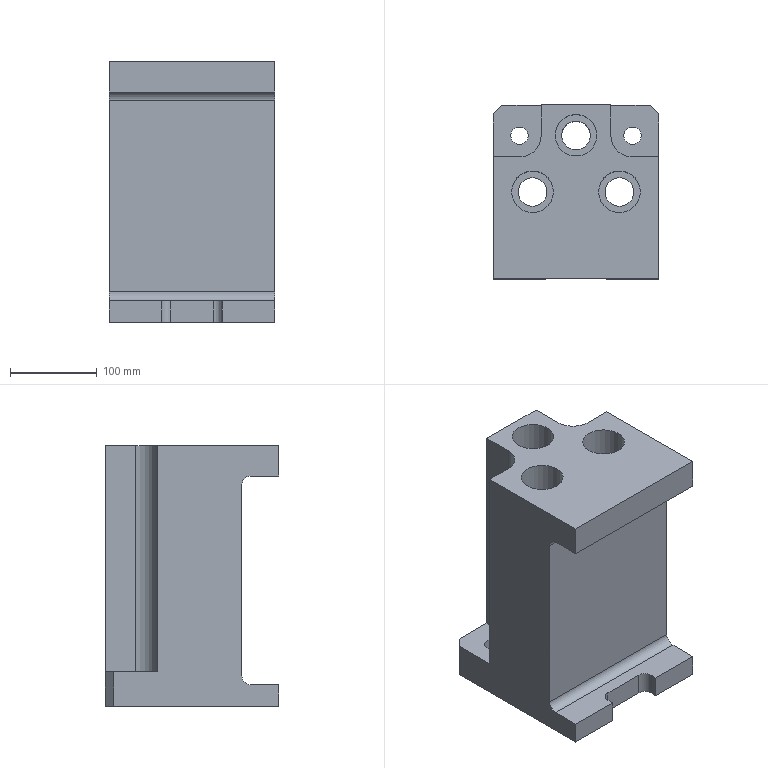Part | NX | features DATUM_CSYS 6, SKETCH 5, EXTRUDE 4, CBORE_HOLE 3, BLEND 2, HOLE PACKAGE 2, SIMPLE HOLE 2, CHAMFER 1 | 1 solid | 39 faces | box 190.5 x 200 x 300 mm | volume 6616630 mm3 | plane 25 | cylinder 14 | commonest cylinder face diameters 20 x6 33 x3 48 x3 50 x2
STEP:
#1=CARTESIAN_POINT('',(-95.25,-100.,0.));
#2=VERTEX_POINT('',#1);
#3=CARTESIAN_POINT('',(-35.,-100.,0.));
#4=VERTEX_POINT('',#3);
#5=CARTESIAN_POINT('',(-95.25,-100.,0.));
#6=DIRECTION('',(1.,0.,0.));
#7=VECTOR('',#6,1000.);
#8=LINE('',#5,#7);
#9=EDGE_CURVE('',#2,#4,#8,.T.);
#10=ORIENTED_EDGE('',*,*,#9,.T.);
#11=CARTESIAN_POINT('',(-35.,-100.,25.));
#12=VERTEX_POINT('',#11);
#13=CARTESIAN_POINT('',(-35.,-100.,300.));
#14=DIRECTION('',(0.,0.,1.));
#15=VECTOR('',#14,1000.);
#16=LINE('',#13,#15);
#17=EDGE_CURVE('',#4,#12,#16,.T.);
#18=ORIENTED_EDGE('',*,*,#17,.T.);
#19=CARTESIAN_POINT('',(-95.25,-100.,25.));
#20=VERTEX_POINT('',#19);
#21=CARTESIAN_POINT('',(-95.25,-100.,25.));
#22=DIRECTION('',(-1.,0.,0.));
#23=VECTOR('',#22,1000.);
#24=LINE('',#21,#23);
#25=EDGE_CURVE('',#12,#20,#24,.T.);
#26=ORIENTED_EDGE('',*,*,#25,.T.);
#27=CARTESIAN_POINT('',(-95.25,-100.,300.));
#28=DIRECTION('',(0.,0.,-1.));
#29=VECTOR('',#28,1000.);
#30=LINE('',#27,#29);
#31=EDGE_CURVE('',#20,#2,#30,.T.);
#32=ORIENTED_EDGE('',*,*,#31,.T.);
#33=EDGE_LOOP('',(#10,#18,#26,#32));
#34=FACE_BOUND('',#33,.T.);
#35=CARTESIAN_POINT('',(-95.25,-100.,300.));
#36=DIRECTION('',(0.,1.,0.));
#37=DIRECTION('',(0.,0.,1.));
#38=AXIS2_PLACEMENT_3D('',#35,#36,#37);
#39=PLANE('',#38);
#40=ADVANCED_FACE('',(#34),#39,.F.);
#41=CARTESIAN_POINT('',(-33.5,0.,0.));
#42=VERTEX_POINT('',#41);
#43=CARTESIAN_POINT('',(-50.,0.,0.));
#44=DIRECTION('',(0.,0.,1.));
#45=DIRECTION('',(1.,0.,0.));
#46=AXIS2_PLACEMENT_3D('',#43,#44,#45);
#47=CIRCLE('',#46,16.5);
#48=EDGE_CURVE('',#42,#42,#47,.T.);
#49=ORIENTED_EDGE('',*,*,#48,.T.);
#50=EDGE_LOOP('',(#49));
#51=FACE_BOUND('',#50,.T.);
#52=CARTESIAN_POINT('',(16.5,65.,0.));
#53=VERTEX_POINT('',#52);
#54=CARTESIAN_POINT('',(0.,65.,0.));
#55=DIRECTION('',(0.,0.,1.));
#56=DIRECTION('',(1.,0.,0.));
#57=AXIS2_PLACEMENT_3D('',#54,#55,#56);
#58=CIRCLE('',#57,16.5);
#59=EDGE_CURVE('',#53,#53,#58,.T.);
#60=ORIENTED_EDGE('',*,*,#59,.T.);
#61=EDGE_LOOP('',(#60));
#62=FACE_BOUND('',#61,.T.);
#63=CARTESIAN_POINT('',(66.5,0.,0.));
#64=VERTEX_POINT('',#63);
#65=CARTESIAN_POINT('',(50.,0.,0.));
#66=DIRECTION('',(0.,0.,1.));
#67=DIRECTION('',(1.,0.,0.));
#68=AXIS2_PLACEMENT_3D('',#65,#66,#67);
#69=CIRCLE('',#68,16.5);
#70=EDGE_CURVE('',#64,#64,#69,.T.);
#71=ORIENTED_EDGE('',*,*,#70,.T.);
#72=EDGE_LOOP('',(#71));
#73=FACE_BOUND('',#72,.T.);
#74=CARTESIAN_POINT('',(-55.,65.,0.));
#75=VERTEX_POINT('',#74);
#76=CARTESIAN_POINT('',(-65.,65.,0.));
#77=DIRECTION('',(0.,0.,1.));
#78=DIRECTION('',(1.,0.,0.));
#79=AXIS2_PLACEMENT_3D('',#76,#77,#78);
#80=CIRCLE('',#79,10.);
#81=EDGE_CURVE('',#75,#75,#80,.T.);
#82=ORIENTED_EDGE('',*,*,#81,.T.);
#83=EDGE_LOOP('',(#82));
#84=FACE_BOUND('',#83,.T.);
#85=CARTESIAN_POINT('',(75.,65.,0.));
#86=VERTEX_POINT('',#85);
#87=CARTESIAN_POINT('',(65.,65.,0.));
#88=DIRECTION('',(0.,0.,1.));
#89=DIRECTION('',(1.,0.,0.));
#90=AXIS2_PLACEMENT_3D('',#87,#88,#89);
#91=CIRCLE('',#90,10.);
#92=EDGE_CURVE('',#86,#86,#91,.T.);
#93=ORIENTED_EDGE('',*,*,#92,.T.);
#94=EDGE_LOOP('',(#93));
#95=FACE_BOUND('',#94,.T.);
#96=CARTESIAN_POINT('',(85.25,100.,0.));
#97=VERTEX_POINT('',#96);
#98=CARTESIAN_POINT('',(-85.25,100.,0.));
#99=VERTEX_POINT('',#98);
#100=CARTESIAN_POINT('',(95.25,100.,0.));
#101=DIRECTION('',(-1.,0.,0.));
#102=VECTOR('',#101,1000.);
#103=LINE('',#100,#102);
#104=EDGE_CURVE('',#97,#99,#103,.T.);
#105=ORIENTED_EDGE('',*,*,#104,.F.);
#106=CARTESIAN_POINT('',(95.25,90.,0.));
#107=VERTEX_POINT('',#106);
#108=CARTESIAN_POINT('',(85.25,100.,0.));
#109=DIRECTION('',(-0.7071,0.7071,0.));
#110=VECTOR('',#109,1000.);
#111=LINE('',#108,#110);
#112=EDGE_CURVE('',#97,#107,#111,.F.);
#113=ORIENTED_EDGE('',*,*,#112,.T.);
#114=CARTESIAN_POINT('',(95.25,-100.,0.));
#115=VERTEX_POINT('',#114);
#116=CARTESIAN_POINT('',(95.25,-100.,0.));
#117=DIRECTION('',(0.,1.,0.));
#118=VECTOR('',#117,1000.);
#119=LINE('',#116,#118);
#120=EDGE_CURVE('',#115,#107,#119,.T.);
#121=ORIENTED_EDGE('',*,*,#120,.F.);
#122=CARTESIAN_POINT('',(35.,-100.,0.));
#123=VERTEX_POINT('',#122);
#124=CARTESIAN_POINT('',(-95.25,-100.,0.));
#125=DIRECTION('',(1.,0.,0.));
#126=VECTOR('',#125,1000.);
#127=LINE('',#124,#126);
#128=EDGE_CURVE('',#123,#115,#127,.T.);
#129=ORIENTED_EDGE('',*,*,#128,.F.);
#130=CARTESIAN_POINT('',(35.,-92.,0.));
#131=VERTEX_POINT('',#130);
#132=CARTESIAN_POINT('',(35.,-82.,0.));
#133=DIRECTION('',(0.,-1.,0.));
#134=VECTOR('',#133,1000.);
#135=LINE('',#132,#134);
#136=EDGE_CURVE('',#131,#123,#135,.T.);
#137=ORIENTED_EDGE('',*,*,#136,.F.);
#138=CARTESIAN_POINT('',(25.,-82.,0.));
#139=VERTEX_POINT('',#138);
#140=CARTESIAN_POINT('',(25.,-92.,0.));
#141=DIRECTION('',(0.,0.,1.));
#142=DIRECTION('',(1.,0.,0.));
#143=AXIS2_PLACEMENT_3D('',#140,#141,#142);
#144=CIRCLE('',#143,10.);
#145=EDGE_CURVE('',#131,#139,#144,.T.);
#146=ORIENTED_EDGE('',*,*,#145,.T.);
#147=CARTESIAN_POINT('',(-25.,-82.,0.));
#148=VERTEX_POINT('',#147);
#149=CARTESIAN_POINT('',(-35.,-82.,0.));
#150=DIRECTION('',(1.,0.,0.));
#151=VECTOR('',#150,1000.);
#152=LINE('',#149,#151);
#153=EDGE_CURVE('',#148,#139,#152,.T.);
#154=ORIENTED_EDGE('',*,*,#153,.F.);
#155=CARTESIAN_POINT('',(-35.,-92.,0.));
#156=VERTEX_POINT('',#155);
#157=CARTESIAN_POINT('',(-25.,-92.,0.));
#158=DIRECTION('',(0.,0.,1.));
#159=DIRECTION('',(1.,0.,0.));
#160=AXIS2_PLACEMENT_3D('',#157,#158,#159);
#161=CIRCLE('',#160,10.);
#162=EDGE_CURVE('',#148,#156,#161,.T.);
#163=ORIENTED_EDGE('',*,*,#162,.T.);
#164=CARTESIAN_POINT('',(-35.,-147.,0.));
#165=DIRECTION('',(0.,1.,0.));
#166=VECTOR('',#165,1000.);
#167=LINE('',#164,#166);
#168=EDGE_CURVE('',#4,#156,#167,.T.);
#169=ORIENTED_EDGE('',*,*,#168,.F.);
#170=ORIENTED_EDGE('',*,*,#9,.F.);
#171=CARTESIAN_POINT('',(-95.25,90.,0.));
#172=VERTEX_POINT('',#171);
#173=CARTESIAN_POINT('',(-95.25,100.,0.));
#174=DIRECTION('',(0.,-1.,0.));
#175=VECTOR('',#174,1000.);
#176=LINE('',#173,#175);
#177=EDGE_CURVE('',#172,#2,#176,.T.);
#178=ORIENTED_EDGE('',*,*,#177,.F.);
#179=CARTESIAN_POINT('',(-95.25,90.,0.));
#180=DIRECTION('',(-0.7071,-0.7071,0.));
#181=VECTOR('',#180,1000.);
#182=LINE('',#179,#181);
#183=EDGE_CURVE('',#172,#99,#182,.F.);
#184=ORIENTED_EDGE('',*,*,#183,.T.);
#185=EDGE_LOOP('',(#105,#113,#121,#129,#137,#146,#154,#163,#169,#170,#178,#184));
#186=FACE_BOUND('',#185,.T.);
#187=CARTESIAN_POINT('',(0.,0.,0.));
#188=DIRECTION('',(0.,0.,1.));
#189=DIRECTION('',(1.,0.,0.));
#190=AXIS2_PLACEMENT_3D('',#187,#188,#189);
#191=PLANE('',#190);
#192=ADVANCED_FACE('',(#51,#62,#73,#84,#95,#186),#191,.F.);
#193=CARTESIAN_POINT('',(95.25,-100.,25.));
#194=VERTEX_POINT('',#193);
#195=CARTESIAN_POINT('',(35.,-100.,25.));
#196=VERTEX_POINT('',#195);
#197=CARTESIAN_POINT('',(-95.25,-100.,25.));
#198=DIRECTION('',(-1.,0.,0.));
#199=VECTOR('',#198,1000.);
#200=LINE('',#197,#199);
#201=EDGE_CURVE('',#194,#196,#200,.T.);
#202=ORIENTED_EDGE('',*,*,#201,.T.);
#203=CARTESIAN_POINT('',(35.,-100.,300.));
#204=DIRECTION('',(0.,0.,-1.));
#205=VECTOR('',#204,1000.);
#206=LINE('',#203,#205);
#207=EDGE_CURVE('',#196,#123,#206,.T.);
#208=ORIENTED_EDGE('',*,*,#207,.T.);
#209=ORIENTED_EDGE('',*,*,#128,.T.);
#210=CARTESIAN_POINT('',(95.25,-100.,300.));
#211=DIRECTION('',(0.,0.,-1.));
#212=VECTOR('',#211,1000.);
#213=LINE('',#210,#212);
#214=EDGE_CURVE('',#194,#115,#213,.T.);
#215=ORIENTED_EDGE('',*,*,#214,.F.);
#216=EDGE_LOOP('',(#202,#208,#209,#215));
#217=FACE_BOUND('',#216,.T.);
#218=CARTESIAN_POINT('',(-95.25,-100.,300.));
#219=DIRECTION('',(0.,1.,0.));
#220=DIRECTION('',(0.,0.,1.));
#221=AXIS2_PLACEMENT_3D('',#218,#219,#220);
#222=PLANE('',#221);
#223=ADVANCED_FACE('',(#217),#222,.F.);
#224=ORIENTED_EDGE('',*,*,#120,.T.);
#225=CARTESIAN_POINT('',(95.25,90.,40.));
#226=VERTEX_POINT('',#225);
#227=CARTESIAN_POINT('',(95.25,90.,300.));
#228=DIRECTION('',(0.,0.,1.));
#229=VECTOR('',#228,1000.);
#230=LINE('',#227,#229);
#231=EDGE_CURVE('',#107,#226,#230,.T.);
#232=ORIENTED_EDGE('',*,*,#231,.T.);
#233=CARTESIAN_POINT('',(95.25,40.,40.));
#234=VERTEX_POINT('',#233);
#235=CARTESIAN_POINT('',(95.25,-100.,40.));
#236=DIRECTION('',(0.,1.,0.));
#237=VECTOR('',#236,1000.);
#238=LINE('',#235,#237);
#239=EDGE_CURVE('',#234,#226,#238,.T.);
#240=ORIENTED_EDGE('',*,*,#239,.F.);
#241=CARTESIAN_POINT('',(95.25,40.,300.));
#242=VERTEX_POINT('',#241);
#243=CARTESIAN_POINT('',(95.25,40.,300.));
#244=DIRECTION('',(0.,0.,1.));
#245=VECTOR('',#244,1000.);
#246=LINE('',#243,#245);
#247=EDGE_CURVE('',#234,#242,#246,.T.);
#248=ORIENTED_EDGE('',*,*,#247,.T.);
#249=CARTESIAN_POINT('',(95.25,-100.,300.));
#250=VERTEX_POINT('',#249);
#251=CARTESIAN_POINT('',(95.25,-100.,300.));
#252=DIRECTION('',(0.,1.,0.));
#253=VECTOR('',#252,1000.);
#254=LINE('',#251,#253);
#255=EDGE_CURVE('',#250,#242,#254,.T.);
#256=ORIENTED_EDGE('',*,*,#255,.F.);
#257=CARTESIAN_POINT('',(95.25,-100.,265.));
#258=VERTEX_POINT('',#257);
#259=CARTESIAN_POINT('',(95.25,-100.,300.));
#260=DIRECTION('',(0.,0.,-1.));
#261=VECTOR('',#260,1000.);
#262=LINE('',#259,#261);
#263=EDGE_CURVE('',#250,#258,#262,.T.);
#264=ORIENTED_EDGE('',*,*,#263,.T.);
#265=CARTESIAN_POINT('',(95.25,-67.5,265.));
#266=VERTEX_POINT('',#265);
#267=CARTESIAN_POINT('',(95.25,-57.5,265.));
#268=DIRECTION('',(0.,-1.,0.));
#269=VECTOR('',#268,1000.);
#270=LINE('',#267,#269);
#271=EDGE_CURVE('',#266,#258,#270,.T.);
#272=ORIENTED_EDGE('',*,*,#271,.F.);
#273=CARTESIAN_POINT('',(95.25,-57.5,255.));
#274=VERTEX_POINT('',#273);
#275=CARTESIAN_POINT('',(95.25,-67.5,255.));
#276=DIRECTION('',(-1.,0.,0.));
#277=DIRECTION('',(0.,-1.,0.));
#278=AXIS2_PLACEMENT_3D('',#275,#276,#277);
#279=CIRCLE('',#278,10.);
#280=EDGE_CURVE('',#266,#274,#279,.T.);
#281=ORIENTED_EDGE('',*,*,#280,.T.);
#282=CARTESIAN_POINT('',(95.25,-57.5,35.));
#283=VERTEX_POINT('',#282);
#284=CARTESIAN_POINT('',(95.25,-57.5,25.));
#285=DIRECTION('',(0.,0.,1.));
#286=VECTOR('',#285,1000.);
#287=LINE('',#284,#286);
#288=EDGE_CURVE('',#283,#274,#287,.T.);
#289=ORIENTED_EDGE('',*,*,#288,.F.);
#290=CARTESIAN_POINT('',(95.25,-67.5,25.));
#291=VERTEX_POINT('',#290);
#292=CARTESIAN_POINT('',(95.25,-67.5,35.));
#293=DIRECTION('',(-1.,0.,0.));
#294=DIRECTION('',(0.,-1.,0.));
#295=AXIS2_PLACEMENT_3D('',#292,#293,#294);
#296=CIRCLE('',#295,10.);
#297=EDGE_CURVE('',#283,#291,#296,.T.);
#298=ORIENTED_EDGE('',*,*,#297,.T.);
#299=CARTESIAN_POINT('',(95.25,-157.5,25.));
#300=DIRECTION('',(0.,1.,0.));
#301=VECTOR('',#300,1000.);
#302=LINE('',#299,#301);
#303=EDGE_CURVE('',#194,#291,#302,.T.);
#304=ORIENTED_EDGE('',*,*,#303,.F.);
#305=ORIENTED_EDGE('',*,*,#214,.T.);
#306=EDGE_LOOP('',(#224,#232,#240,#248,#256,#264,#272,#281,#289,#298,#304,#305));
#307=FACE_BOUND('',#306,.T.);
#308=CARTESIAN_POINT('',(95.25,-100.,300.));
#309=DIRECTION('',(-1.,0.,0.));
#310=DIRECTION('',(0.,-1.,0.));
#311=AXIS2_PLACEMENT_3D('',#308,#309,#310);
#312=PLANE('',#311);
#313=ADVANCED_FACE('',(#307),#312,.F.);
#314=CARTESIAN_POINT('',(-95.25,90.,40.));
#315=VERTEX_POINT('',#314);
#316=CARTESIAN_POINT('',(-95.25,40.,40.));
#317=VERTEX_POINT('',#316);
#318=CARTESIAN_POINT('',(-95.25,100.,40.));
#319=DIRECTION('',(0.,-1.,0.));
#320=VECTOR('',#319,1000.);
#321=LINE('',#318,#320);
#322=EDGE_CURVE('',#315,#317,#321,.T.);
#323=ORIENTED_EDGE('',*,*,#322,.F.);
#324=CARTESIAN_POINT('',(-95.25,90.,300.));
#325=DIRECTION('',(0.,0.,-1.));
#326=VECTOR('',#325,1000.);
#327=LINE('',#324,#326);
#328=EDGE_CURVE('',#315,#172,#327,.T.);
#329=ORIENTED_EDGE('',*,*,#328,.T.);
#330=ORIENTED_EDGE('',*,*,#177,.T.);
#331=ORIENTED_EDGE('',*,*,#31,.F.);
#332=CARTESIAN_POINT('',(-95.25,-67.5,25.));
#333=VERTEX_POINT('',#332);
#334=CARTESIAN_POINT('',(-95.25,100.,25.));
#335=DIRECTION('',(0.,1.,0.));
#336=VECTOR('',#335,1000.);
#337=LINE('',#334,#336);
#338=EDGE_CURVE('',#20,#333,#337,.T.);
#339=ORIENTED_EDGE('',*,*,#338,.T.);
#340=CARTESIAN_POINT('',(-95.25,-57.5,35.));
#341=VERTEX_POINT('',#340);
#342=CARTESIAN_POINT('',(-95.25,-67.5,35.));
#343=DIRECTION('',(1.,0.,0.));
#344=DIRECTION('',(0.,1.,0.));
#345=AXIS2_PLACEMENT_3D('',#342,#343,#344);
#346=CIRCLE('',#345,10.);
#347=EDGE_CURVE('',#333,#341,#346,.T.);
#348=ORIENTED_EDGE('',*,*,#347,.T.);
#349=CARTESIAN_POINT('',(-95.25,-57.5,255.));
#350=VERTEX_POINT('',#349);
#351=CARTESIAN_POINT('',(-95.25,-57.5,300.));
#352=DIRECTION('',(0.,0.,1.));
#353=VECTOR('',#352,1000.);
#354=LINE('',#351,#353);
#355=EDGE_CURVE('',#341,#350,#354,.T.);
#356=ORIENTED_EDGE('',*,*,#355,.T.);
#357=CARTESIAN_POINT('',(-95.25,-67.5,265.));
#358=VERTEX_POINT('',#357);
#359=CARTESIAN_POINT('',(-95.25,-67.5,255.));
#360=DIRECTION('',(1.,0.,0.));
#361=DIRECTION('',(0.,1.,0.));
#362=AXIS2_PLACEMENT_3D('',#359,#360,#361);
#363=CIRCLE('',#362,10.);
#364=EDGE_CURVE('',#350,#358,#363,.T.);
#365=ORIENTED_EDGE('',*,*,#364,.T.);
#366=CARTESIAN_POINT('',(-95.25,-100.,265.));
#367=VERTEX_POINT('',#366);
#368=CARTESIAN_POINT('',(-95.25,100.,265.));
#369=DIRECTION('',(0.,-1.,0.));
#370=VECTOR('',#369,1000.);
#371=LINE('',#368,#370);
#372=EDGE_CURVE('',#358,#367,#371,.T.);
#373=ORIENTED_EDGE('',*,*,#372,.T.);
#374=CARTESIAN_POINT('',(-95.25,-100.,300.));
#375=VERTEX_POINT('',#374);
#376=CARTESIAN_POINT('',(-95.25,-100.,300.));
#377=DIRECTION('',(0.,0.,-1.));
#378=VECTOR('',#377,1000.);
#379=LINE('',#376,#378);
#380=EDGE_CURVE('',#375,#367,#379,.T.);
#381=ORIENTED_EDGE('',*,*,#380,.F.);
#382=CARTESIAN_POINT('',(-95.25,40.,300.));
#383=VERTEX_POINT('',#382);
#384=CARTESIAN_POINT('',(-95.25,100.,300.));
#385=DIRECTION('',(0.,-1.,0.));
#386=VECTOR('',#385,1000.);
#387=LINE('',#384,#386);
#388=EDGE_CURVE('',#383,#375,#387,.T.);
#389=ORIENTED_EDGE('',*,*,#388,.F.);
#390=CARTESIAN_POINT('',(-95.25,40.,300.));
#391=DIRECTION('',(0.,0.,-1.));
#392=VECTOR('',#391,1000.);
#393=LINE('',#390,#392);
#394=EDGE_CURVE('',#383,#317,#393,.T.);
#395=ORIENTED_EDGE('',*,*,#394,.T.);
#396=EDGE_LOOP('',(#323,#329,#330,#331,#339,#348,#356,#365,#373,#381,#389,#395));
#397=FACE_BOUND('',#396,.T.);
#398=CARTESIAN_POINT('',(-95.25,100.,300.));
#399=DIRECTION('',(1.,0.,0.));
#400=DIRECTION('',(0.,1.,0.));
#401=AXIS2_PLACEMENT_3D('',#398,#399,#400);
#402=PLANE('',#401);
#403=ADVANCED_FACE('',(#397),#402,.F.);
#404=ORIENTED_EDGE('',*,*,#380,.T.);
#405=CARTESIAN_POINT('',(-95.25,-100.,265.));
#406=DIRECTION('',(1.,0.,0.));
#407=VECTOR('',#406,1000.);
#408=LINE('',#405,#407);
#409=EDGE_CURVE('',#367,#258,#408,.T.);
#410=ORIENTED_EDGE('',*,*,#409,.T.);
#411=ORIENTED_EDGE('',*,*,#263,.F.);
#412=CARTESIAN_POINT('',(-95.25,-100.,300.));
#413=DIRECTION('',(1.,0.,0.));
#414=VECTOR('',#413,1000.);
#415=LINE('',#412,#414);
#416=EDGE_CURVE('',#375,#250,#415,.T.);
#417=ORIENTED_EDGE('',*,*,#416,.F.);
#418=EDGE_LOOP('',(#404,#410,#411,#417));
#419=FACE_BOUND('',#418,.T.);
#420=CARTESIAN_POINT('',(-95.25,-100.,300.));
#421=DIRECTION('',(0.,1.,0.));
#422=DIRECTION('',(0.,0.,1.));
#423=AXIS2_PLACEMENT_3D('',#420,#421,#422);
#424=PLANE('',#423);
#425=ADVANCED_FACE('',(#419),#424,.F.);
#426=CARTESIAN_POINT('',(85.25,100.,40.));
#427=VERTEX_POINT('',#426);
#428=CARTESIAN_POINT('',(40.,100.,40.));
#429=VERTEX_POINT('',#428);
#430=CARTESIAN_POINT('',(95.25,100.,40.));
#431=DIRECTION('',(-1.,0.,0.));
#432=VECTOR('',#431,1000.);
#433=LINE('',#430,#432);
#434=EDGE_CURVE('',#427,#429,#433,.T.);
#435=ORIENTED_EDGE('',*,*,#434,.F.);
#436=CARTESIAN_POINT('',(85.25,100.,300.));
#437=DIRECTION('',(0.,0.,-1.));
#438=VECTOR('',#437,1000.);
#439=LINE('',#436,#438);
#440=EDGE_CURVE('',#427,#97,#439,.T.);
#441=ORIENTED_EDGE('',*,*,#440,.T.);
#442=ORIENTED_EDGE('',*,*,#104,.T.);
#443=CARTESIAN_POINT('',(-85.25,100.,40.));
#444=VERTEX_POINT('',#443);
#445=CARTESIAN_POINT('',(-85.25,100.,300.));
#446=DIRECTION('',(0.,0.,1.));
#447=VECTOR('',#446,1000.);
#448=LINE('',#445,#447);
#449=EDGE_CURVE('',#99,#444,#448,.T.);
#450=ORIENTED_EDGE('',*,*,#449,.T.);
#451=CARTESIAN_POINT('',(-40.,100.,40.));
#452=VERTEX_POINT('',#451);
#453=CARTESIAN_POINT('',(95.25,100.,40.));
#454=DIRECTION('',(-1.,0.,0.));
#455=VECTOR('',#454,1000.);
#456=LINE('',#453,#455);
#457=EDGE_CURVE('',#452,#444,#456,.T.);
#458=ORIENTED_EDGE('',*,*,#457,.F.);
#459=CARTESIAN_POINT('',(-40.,100.,300.));
#460=VERTEX_POINT('',#459);
#461=CARTESIAN_POINT('',(-40.,100.,300.));
#462=DIRECTION('',(0.,0.,1.));
#463=VECTOR('',#462,1000.);
#464=LINE('',#461,#463);
#465=EDGE_CURVE('',#452,#460,#464,.T.);
#466=ORIENTED_EDGE('',*,*,#465,.T.);
#467=CARTESIAN_POINT('',(40.,100.,300.));
#468=VERTEX_POINT('',#467);
#469=CARTESIAN_POINT('',(95.25,100.,300.));
#470=DIRECTION('',(-1.,0.,0.));
#471=VECTOR('',#470,1000.);
#472=LINE('',#469,#471);
#473=EDGE_CURVE('',#468,#460,#472,.T.);
#474=ORIENTED_EDGE('',*,*,#473,.F.);
#475=CARTESIAN_POINT('',(40.,100.,300.));
#476=DIRECTION('',(0.,0.,-1.));
#477=VECTOR('',#476,1000.);
#478=LINE('',#475,#477);
#479=EDGE_CURVE('',#468,#429,#478,.T.);
#480=ORIENTED_EDGE('',*,*,#479,.T.);
#481=EDGE_LOOP('',(#435,#441,#442,#450,#458,#466,#474,#480));
#482=FACE_BOUND('',#481,.T.);
#483=CARTESIAN_POINT('',(95.25,100.,300.));
#484=DIRECTION('',(0.,-1.,0.));
#485=DIRECTION('',(0.,0.,-1.));
#486=AXIS2_PLACEMENT_3D('',#483,#484,#485);
#487=PLANE('',#486);
#488=ADVANCED_FACE('',(#482),#487,.F.);
#489=CARTESIAN_POINT('',(26.,0.,300.));
#490=VERTEX_POINT('',#489);
#491=CARTESIAN_POINT('',(50.,0.,300.));
#492=DIRECTION('',(0.,0.,-1.));
#493=DIRECTION('',(-1.,0.,0.));
#494=AXIS2_PLACEMENT_3D('',#491,#492,#493);
#495=CIRCLE('',#494,24.);
#496=EDGE_CURVE('',#490,#490,#495,.T.);
#497=ORIENTED_EDGE('',*,*,#496,.T.);
#498=EDGE_LOOP('',(#497));
#499=FACE_BOUND('',#498,.T.);
#500=CARTESIAN_POINT('',(-24.,65.,300.));
#501=VERTEX_POINT('',#500);
#502=CARTESIAN_POINT('',(0.,65.,300.));
#503=DIRECTION('',(0.,0.,-1.));
#504=DIRECTION('',(-1.,0.,0.));
#505=AXIS2_PLACEMENT_3D('',#502,#503,#504);
#506=CIRCLE('',#505,24.);
#507=EDGE_CURVE('',#501,#501,#506,.T.);
#508=ORIENTED_EDGE('',*,*,#507,.T.);
#509=EDGE_LOOP('',(#508));
#510=FACE_BOUND('',#509,.T.);
#511=CARTESIAN_POINT('',(-74.,0.,300.));
#512=VERTEX_POINT('',#511);
#513=CARTESIAN_POINT('',(-50.,0.,300.));
#514=DIRECTION('',(0.,0.,-1.));
#515=DIRECTION('',(-1.,0.,0.));
#516=AXIS2_PLACEMENT_3D('',#513,#514,#515);
#517=CIRCLE('',#516,24.);
#518=EDGE_CURVE('',#512,#512,#517,.T.);
#519=ORIENTED_EDGE('',*,*,#518,.T.);
#520=EDGE_LOOP('',(#519));
#521=FACE_BOUND('',#520,.T.);
#522=CARTESIAN_POINT('',(40.,65.,300.));
#523=VERTEX_POINT('',#522);
#524=CARTESIAN_POINT('',(40.,134.638,300.));
#525=DIRECTION('',(0.,-1.,0.));
#526=VECTOR('',#525,1000.);
#527=LINE('',#524,#526);
#528=EDGE_CURVE('',#468,#523,#527,.T.);
#529=ORIENTED_EDGE('',*,*,#528,.F.);
#530=ORIENTED_EDGE('',*,*,#473,.T.);
#531=CARTESIAN_POINT('',(-40.,65.,300.));
#532=VERTEX_POINT('',#531);
#533=CARTESIAN_POINT('',(-40.,65.,300.));
#534=DIRECTION('',(0.,1.,0.));
#535=VECTOR('',#534,1000.);
#536=LINE('',#533,#535);
#537=EDGE_CURVE('',#532,#460,#536,.T.);
#538=ORIENTED_EDGE('',*,*,#537,.F.);
#539=CARTESIAN_POINT('',(-65.,40.,300.));
#540=VERTEX_POINT('',#539);
#541=CARTESIAN_POINT('',(-65.,65.,300.));
#542=DIRECTION('',(0.,0.,1.));
#543=DIRECTION('',(1.,0.,0.));
#544=AXIS2_PLACEMENT_3D('',#541,#542,#543);
#545=CIRCLE('',#544,25.);
#546=EDGE_CURVE('',#540,#532,#545,.T.);
#547=ORIENTED_EDGE('',*,*,#546,.F.);
#548=CARTESIAN_POINT('',(-158.968,40.,300.));
#549=DIRECTION('',(1.,0.,0.));
#550=VECTOR('',#549,1000.);
#551=LINE('',#548,#550);
#552=EDGE_CURVE('',#383,#540,#551,.T.);
#553=ORIENTED_EDGE('',*,*,#552,.F.);
#554=ORIENTED_EDGE('',*,*,#388,.T.);
#555=ORIENTED_EDGE('',*,*,#416,.T.);
#556=ORIENTED_EDGE('',*,*,#255,.T.);
#557=CARTESIAN_POINT('',(65.,40.,300.));
#558=VERTEX_POINT('',#557);
#559=CARTESIAN_POINT('',(65.,40.,300.));
#560=DIRECTION('',(1.,0.,0.));
#561=VECTOR('',#560,1000.);
#562=LINE('',#559,#561);
#563=EDGE_CURVE('',#558,#242,#562,.T.);
#564=ORIENTED_EDGE('',*,*,#563,.F.);
#565=CARTESIAN_POINT('',(65.,65.,300.));
#566=DIRECTION('',(0.,0.,1.));
#567=DIRECTION('',(1.,0.,0.));
#568=AXIS2_PLACEMENT_3D('',#565,#566,#567);
#569=CIRCLE('',#568,25.);
#570=EDGE_CURVE('',#523,#558,#569,.T.);
#571=ORIENTED_EDGE('',*,*,#570,.F.);
#572=EDGE_LOOP('',(#529,#530,#538,#547,#553,#554,#555,#556,#564,#571));
#573=FACE_BOUND('',#572,.T.);
#574=CARTESIAN_POINT('',(0.,0.,300.));
#575=DIRECTION('',(0.,0.,1.));
#576=DIRECTION('',(1.,0.,0.));
#577=AXIS2_PLACEMENT_3D('',#574,#575,#576);
#578=PLANE('',#577);
#579=ADVANCED_FACE('',(#499,#510,#521,#573),#578,.T.);
#580=ORIENTED_EDGE('',*,*,#552,.T.);
#581=CARTESIAN_POINT('',(-65.,40.,40.));
#582=VERTEX_POINT('',#581);
#583=CARTESIAN_POINT('',(-65.,40.,40.));
#584=DIRECTION('',(0.,0.,1.));
#585=VECTOR('',#584,1000.);
#586=LINE('',#583,#585);
#587=EDGE_CURVE('',#540,#582,#586,.F.);
#588=ORIENTED_EDGE('',*,*,#587,.T.);
#589=CARTESIAN_POINT('',(-158.968,40.,40.));
#590=DIRECTION('',(1.,0.,0.));
#591=VECTOR('',#590,1000.);
#592=LINE('',#589,#591);
#593=EDGE_CURVE('',#582,#317,#592,.F.);
#594=ORIENTED_EDGE('',*,*,#593,.T.);
#595=ORIENTED_EDGE('',*,*,#394,.F.);
#596=EDGE_LOOP('',(#580,#588,#594,#595));
#597=FACE_BOUND('',#596,.T.);
#598=CARTESIAN_POINT('',(-158.968,40.,40.));
#599=DIRECTION('',(0.,-1.,0.));
#600=DIRECTION('',(0.,0.,-1.));
#601=AXIS2_PLACEMENT_3D('',#598,#599,#600);
#602=PLANE('',#601);
#603=ADVANCED_FACE('',(#597),#602,.F.);
#604=CARTESIAN_POINT('',(-40.,65.,40.));
#605=VERTEX_POINT('',#604);
#606=CARTESIAN_POINT('',(-40.,65.,40.));
#607=DIRECTION('',(0.,1.,0.));
#608=VECTOR('',#607,1000.);
#609=LINE('',#606,#608);
#610=EDGE_CURVE('',#452,#605,#609,.F.);
#611=ORIENTED_EDGE('',*,*,#610,.T.);
#612=CARTESIAN_POINT('',(-40.,65.,40.));
#613=DIRECTION('',(0.,0.,1.));
#614=VECTOR('',#613,1000.);
#615=LINE('',#612,#614);
#616=EDGE_CURVE('',#532,#605,#615,.F.);
#617=ORIENTED_EDGE('',*,*,#616,.F.);
#618=ORIENTED_EDGE('',*,*,#537,.T.);
#619=ORIENTED_EDGE('',*,*,#465,.F.);
#620=EDGE_LOOP('',(#611,#617,#618,#619));
#621=FACE_BOUND('',#620,.T.);
#622=CARTESIAN_POINT('',(-40.,65.,40.));
#623=DIRECTION('',(1.,0.,0.));
#624=DIRECTION('',(0.,0.,-1.));
#625=AXIS2_PLACEMENT_3D('',#622,#623,#624);
#626=PLANE('',#625);
#627=ADVANCED_FACE('',(#621),#626,.F.);
#628=CARTESIAN_POINT('',(-75.,65.,40.));
#629=VERTEX_POINT('',#628);
#630=CARTESIAN_POINT('',(-65.,65.,40.));
#631=DIRECTION('',(0.,0.,-1.));
#632=DIRECTION('',(-1.,0.,0.));
#633=AXIS2_PLACEMENT_3D('',#630,#631,#632);
#634=CIRCLE('',#633,10.);
#635=EDGE_CURVE('',#629,#629,#634,.T.);
#636=ORIENTED_EDGE('',*,*,#635,.T.);
#637=EDGE_LOOP('',(#636));
#638=FACE_BOUND('',#637,.T.);
#639=ORIENTED_EDGE('',*,*,#457,.T.);
#640=CARTESIAN_POINT('',(-92.625,92.625,40.));
#641=DIRECTION('',(0.7071,0.7071,0.));
#642=VECTOR('',#641,1000.);
#643=LINE('',#640,#642);
#644=EDGE_CURVE('',#444,#315,#643,.F.);
#645=ORIENTED_EDGE('',*,*,#644,.T.);
#646=ORIENTED_EDGE('',*,*,#322,.T.);
#647=ORIENTED_EDGE('',*,*,#593,.F.);
#648=CARTESIAN_POINT('',(-65.,65.,40.));
#649=DIRECTION('',(0.,0.,1.));
#650=DIRECTION('',(1.,0.,0.));
#651=AXIS2_PLACEMENT_3D('',#648,#649,#650);
#652=CIRCLE('',#651,25.);
#653=EDGE_CURVE('',#605,#582,#652,.F.);
#654=ORIENTED_EDGE('',*,*,#653,.F.);
#655=ORIENTED_EDGE('',*,*,#610,.F.);
#656=EDGE_LOOP('',(#639,#645,#646,#647,#654,#655));
#657=FACE_BOUND('',#656,.T.);
#658=CARTESIAN_POINT('',(-65.,65.,40.));
#659=DIRECTION('',(0.,0.,1.));
#660=DIRECTION('',(1.,0.,0.));
#661=AXIS2_PLACEMENT_3D('',#658,#659,#660);
#662=PLANE('',#661);
#663=ADVANCED_FACE('',(#638,#657),#662,.T.);
#664=ORIENTED_EDGE('',*,*,#546,.T.);
#665=ORIENTED_EDGE('',*,*,#616,.T.);
#666=ORIENTED_EDGE('',*,*,#653,.T.);
#667=ORIENTED_EDGE('',*,*,#587,.F.);
#668=EDGE_LOOP('',(#664,#665,#666,#667));
#669=FACE_BOUND('',#668,.T.);
#670=CARTESIAN_POINT('',(-65.,65.,40.));
#671=DIRECTION('',(0.,0.,1.));
#672=DIRECTION('',(1.,0.,0.));
#673=AXIS2_PLACEMENT_3D('',#670,#671,#672);
#674=CYLINDRICAL_SURFACE('',#673,25.);
#675=ADVANCED_FACE('',(#669),#674,.F.);
#676=CARTESIAN_POINT('',(65.,40.,40.));
#677=VERTEX_POINT('',#676);
#678=CARTESIAN_POINT('',(65.,40.,40.));
#679=DIRECTION('',(1.,0.,0.));
#680=VECTOR('',#679,1000.);
#681=LINE('',#678,#680);
#682=EDGE_CURVE('',#234,#677,#681,.F.);
#683=ORIENTED_EDGE('',*,*,#682,.T.);
#684=CARTESIAN_POINT('',(65.,40.,40.));
#685=DIRECTION('',(0.,0.,1.));
#686=VECTOR('',#685,1000.);
#687=LINE('',#684,#686);
#688=EDGE_CURVE('',#558,#677,#687,.F.);
#689=ORIENTED_EDGE('',*,*,#688,.F.);
#690=ORIENTED_EDGE('',*,*,#563,.T.);
#691=ORIENTED_EDGE('',*,*,#247,.F.);
#692=EDGE_LOOP('',(#683,#689,#690,#691));
#693=FACE_BOUND('',#692,.T.);
#694=CARTESIAN_POINT('',(65.,40.,40.));
#695=DIRECTION('',(0.,-1.,0.));
#696=DIRECTION('',(0.,0.,-1.));
#697=AXIS2_PLACEMENT_3D('',#694,#695,#696);
#698=PLANE('',#697);
#699=ADVANCED_FACE('',(#693),#698,.F.);
#700=ORIENTED_EDGE('',*,*,#528,.T.);
#701=CARTESIAN_POINT('',(40.,65.,40.));
#702=VERTEX_POINT('',#701);
#703=CARTESIAN_POINT('',(40.,65.,40.));
#704=DIRECTION('',(0.,0.,1.));
#705=VECTOR('',#704,1000.);
#706=LINE('',#703,#705);
#707=EDGE_CURVE('',#523,#702,#706,.F.);
#708=ORIENTED_EDGE('',*,*,#707,.T.);
#709=CARTESIAN_POINT('',(40.,134.638,40.));
#710=DIRECTION('',(0.,-1.,0.));
#711=VECTOR('',#710,1000.);
#712=LINE('',#709,#711);
#713=EDGE_CURVE('',#702,#429,#712,.F.);
#714=ORIENTED_EDGE('',*,*,#713,.T.);
#715=ORIENTED_EDGE('',*,*,#479,.F.);
#716=EDGE_LOOP('',(#700,#708,#714,#715));
#717=FACE_BOUND('',#716,.T.);
#718=CARTESIAN_POINT('',(40.,134.638,40.));
#719=DIRECTION('',(-1.,0.,0.));
#720=DIRECTION('',(0.,0.,1.));
#721=AXIS2_PLACEMENT_3D('',#718,#719,#720);
#722=PLANE('',#721);
#723=ADVANCED_FACE('',(#717),#722,.F.);
#724=CARTESIAN_POINT('',(55.,65.,40.));
#725=VERTEX_POINT('',#724);
#726=CARTESIAN_POINT('',(65.,65.,40.));
#727=DIRECTION('',(0.,0.,-1.));
#728=DIRECTION('',(-1.,0.,0.));
#729=AXIS2_PLACEMENT_3D('',#726,#727,#728);
#730=CIRCLE('',#729,10.);
#731=EDGE_CURVE('',#725,#725,#730,.T.);
#732=ORIENTED_EDGE('',*,*,#731,.T.);
#733=EDGE_LOOP('',(#732));
#734=FACE_BOUND('',#733,.T.);
#735=ORIENTED_EDGE('',*,*,#239,.T.);
#736=CARTESIAN_POINT('',(92.625,92.625,40.));
#737=DIRECTION('',(0.7071,-0.7071,0.));
#738=VECTOR('',#737,1000.);
#739=LINE('',#736,#738);
#740=EDGE_CURVE('',#226,#427,#739,.F.);
#741=ORIENTED_EDGE('',*,*,#740,.T.);
#742=ORIENTED_EDGE('',*,*,#434,.T.);
#743=ORIENTED_EDGE('',*,*,#713,.F.);
#744=CARTESIAN_POINT('',(65.,65.,40.));
#745=DIRECTION('',(0.,0.,1.));
#746=DIRECTION('',(1.,0.,0.));
#747=AXIS2_PLACEMENT_3D('',#744,#745,#746);
#748=CIRCLE('',#747,25.);
#749=EDGE_CURVE('',#677,#702,#748,.F.);
#750=ORIENTED_EDGE('',*,*,#749,.F.);
#751=ORIENTED_EDGE('',*,*,#682,.F.);
#752=EDGE_LOOP('',(#735,#741,#742,#743,#750,#751));
#753=FACE_BOUND('',#752,.T.);
#754=CARTESIAN_POINT('',(65.,65.,40.));
#755=DIRECTION('',(0.,0.,1.));
#756=DIRECTION('',(1.,0.,0.));
#757=AXIS2_PLACEMENT_3D('',#754,#755,#756);
#758=PLANE('',#757);
#759=ADVANCED_FACE('',(#734,#753),#758,.T.);
#760=ORIENTED_EDGE('',*,*,#570,.T.);
#761=ORIENTED_EDGE('',*,*,#688,.T.);
#762=ORIENTED_EDGE('',*,*,#749,.T.);
#763=ORIENTED_EDGE('',*,*,#707,.F.);
#764=EDGE_LOOP('',(#760,#761,#762,#763));
#765=FACE_BOUND('',#764,.T.);
#766=CARTESIAN_POINT('',(65.,65.,40.));
#767=DIRECTION('',(0.,0.,1.));
#768=DIRECTION('',(1.,0.,0.));
#769=AXIS2_PLACEMENT_3D('',#766,#767,#768);
#770=CYLINDRICAL_SURFACE('',#769,25.);
#771=ADVANCED_FACE('',(#765),#770,.F.);
#772=CARTESIAN_POINT('',(-66.5,0.,162.));
#773=VERTEX_POINT('',#772);
#774=CARTESIAN_POINT('',(-50.,0.,162.));
#775=DIRECTION('',(0.,0.,-1.));
#776=DIRECTION('',(-1.,0.,0.));
#777=AXIS2_PLACEMENT_3D('',#774,#775,#776);
#778=CIRCLE('',#777,16.5);
#779=EDGE_CURVE('',#773,#773,#778,.F.);
#780=ORIENTED_EDGE('',*,*,#779,.T.);
#781=EDGE_LOOP('',(#780));
#782=FACE_BOUND('',#781,.T.);
#783=ORIENTED_EDGE('',*,*,#48,.F.);
#784=EDGE_LOOP('',(#783));
#785=FACE_BOUND('',#784,.T.);
#786=CARTESIAN_POINT('',(-50.,0.,-50.));
#787=DIRECTION('',(0.,0.,-1.));
#788=DIRECTION('',(-1.,0.,0.));
#789=AXIS2_PLACEMENT_3D('',#786,#787,#788);
#790=CYLINDRICAL_SURFACE('',#789,16.5);
#791=ADVANCED_FACE('',(#782,#785),#790,.F.);
#792=ORIENTED_EDGE('',*,*,#779,.F.);
#793=EDGE_LOOP('',(#792));
#794=FACE_BOUND('',#793,.T.);
#795=CARTESIAN_POINT('',(-74.,0.,162.));
#796=VERTEX_POINT('',#795);
#797=CARTESIAN_POINT('',(-50.,0.,162.));
#798=DIRECTION('',(0.,0.,-1.));
#799=DIRECTION('',(-1.,0.,0.));
#800=AXIS2_PLACEMENT_3D('',#797,#798,#799);
#801=CIRCLE('',#800,24.);
#802=EDGE_CURVE('',#796,#796,#801,.F.);
#803=ORIENTED_EDGE('',*,*,#802,.T.);
#804=EDGE_LOOP('',(#803));
#805=FACE_BOUND('',#804,.T.);
#806=CARTESIAN_POINT('',(-50.,0.,162.));
#807=DIRECTION('',(0.,0.,-1.));
#808=DIRECTION('',(-1.,0.,0.));
#809=AXIS2_PLACEMENT_3D('',#806,#807,#808);
#810=PLANE('',#809);
#811=ADVANCED_FACE('',(#794,#805),#810,.F.);
#812=ORIENTED_EDGE('',*,*,#802,.F.);
#813=EDGE_LOOP('',(#812));
#814=FACE_BOUND('',#813,.T.);
#815=ORIENTED_EDGE('',*,*,#518,.F.);
#816=EDGE_LOOP('',(#815));
#817=FACE_BOUND('',#816,.T.);
#818=CARTESIAN_POINT('',(-50.,0.,300.));
#819=DIRECTION('',(0.,0.,-1.));
#820=DIRECTION('',(-1.,0.,0.));
#821=AXIS2_PLACEMENT_3D('',#818,#819,#820);
#822=CYLINDRICAL_SURFACE('',#821,24.);
#823=ADVANCED_FACE('',(#814,#817),#822,.F.);
#824=CARTESIAN_POINT('',(-16.5,65.,162.));
#825=VERTEX_POINT('',#824);
#826=CARTESIAN_POINT('',(0.,65.,162.));
#827=DIRECTION('',(0.,0.,-1.));
#828=DIRECTION('',(-1.,0.,0.));
#829=AXIS2_PLACEMENT_3D('',#826,#827,#828);
#830=CIRCLE('',#829,16.5);
#831=EDGE_CURVE('',#825,#825,#830,.F.);
#832=ORIENTED_EDGE('',*,*,#831,.T.);
#833=EDGE_LOOP('',(#832));
#834=FACE_BOUND('',#833,.T.);
#835=ORIENTED_EDGE('',*,*,#59,.F.);
#836=EDGE_LOOP('',(#835));
#837=FACE_BOUND('',#836,.T.);
#838=CARTESIAN_POINT('',(0.,65.,-50.));
#839=DIRECTION('',(0.,0.,-1.));
#840=DIRECTION('',(-1.,0.,0.));
#841=AXIS2_PLACEMENT_3D('',#838,#839,#840);
#842=CYLINDRICAL_SURFACE('',#841,16.5);
#843=ADVANCED_FACE('',(#834,#837),#842,.F.);
#844=ORIENTED_EDGE('',*,*,#831,.F.);
#845=EDGE_LOOP('',(#844));
#846=FACE_BOUND('',#845,.T.);
#847=CARTESIAN_POINT('',(-24.,65.,162.));
#848=VERTEX_POINT('',#847);
#849=CARTESIAN_POINT('',(0.,65.,162.));
#850=DIRECTION('',(0.,0.,-1.));
#851=DIRECTION('',(-1.,0.,0.));
#852=AXIS2_PLACEMENT_3D('',#849,#850,#851);
#853=CIRCLE('',#852,24.);
#854=EDGE_CURVE('',#848,#848,#853,.F.);
#855=ORIENTED_EDGE('',*,*,#854,.T.);
#856=EDGE_LOOP('',(#855));
#857=FACE_BOUND('',#856,.T.);
#858=CARTESIAN_POINT('',(0.,65.,162.));
#859=DIRECTION('',(0.,0.,-1.));
#860=DIRECTION('',(-1.,0.,0.));
#861=AXIS2_PLACEMENT_3D('',#858,#859,#860);
#862=PLANE('',#861);
#863=ADVANCED_FACE('',(#846,#857),#862,.F.);
#864=ORIENTED_EDGE('',*,*,#854,.F.);
#865=EDGE_LOOP('',(#864));
#866=FACE_BOUND('',#865,.T.);
#867=ORIENTED_EDGE('',*,*,#507,.F.);
#868=EDGE_LOOP('',(#867));
#869=FACE_BOUND('',#868,.T.);
#870=CARTESIAN_POINT('',(0.,65.,300.));
#871=DIRECTION('',(0.,0.,-1.));
#872=DIRECTION('',(-1.,0.,0.));
#873=AXIS2_PLACEMENT_3D('',#870,#871,#872);
#874=CYLINDRICAL_SURFACE('',#873,24.);
#875=ADVANCED_FACE('',(#866,#869),#874,.F.);
#876=CARTESIAN_POINT('',(33.5,0.,162.));
#877=VERTEX_POINT('',#876);
#878=CARTESIAN_POINT('',(50.,0.,162.));
#879=DIRECTION('',(0.,0.,-1.));
#880=DIRECTION('',(-1.,0.,0.));
#881=AXIS2_PLACEMENT_3D('',#878,#879,#880);
#882=CIRCLE('',#881,16.5);
#883=EDGE_CURVE('',#877,#877,#882,.F.);
#884=ORIENTED_EDGE('',*,*,#883,.T.);
#885=EDGE_LOOP('',(#884));
#886=FACE_BOUND('',#885,.T.);
#887=ORIENTED_EDGE('',*,*,#70,.F.);
#888=EDGE_LOOP('',(#887));
#889=FACE_BOUND('',#888,.T.);
#890=CARTESIAN_POINT('',(50.,0.,-50.));
#891=DIRECTION('',(0.,0.,-1.));
#892=DIRECTION('',(-1.,0.,0.));
#893=AXIS2_PLACEMENT_3D('',#890,#891,#892);
#894=CYLINDRICAL_SURFACE('',#893,16.5);
#895=ADVANCED_FACE('',(#886,#889),#894,.F.);
#896=ORIENTED_EDGE('',*,*,#883,.F.);
#897=EDGE_LOOP('',(#896));
#898=FACE_BOUND('',#897,.T.);
#899=CARTESIAN_POINT('',(26.,0.,162.));
#900=VERTEX_POINT('',#899);
#901=CARTESIAN_POINT('',(50.,0.,162.));
#902=DIRECTION('',(0.,0.,-1.));
#903=DIRECTION('',(-1.,0.,0.));
#904=AXIS2_PLACEMENT_3D('',#901,#902,#903);
#905=CIRCLE('',#904,24.);
#906=EDGE_CURVE('',#900,#900,#905,.F.);
#907=ORIENTED_EDGE('',*,*,#906,.T.);
#908=EDGE_LOOP('',(#907));
#909=FACE_BOUND('',#908,.T.);
#910=CARTESIAN_POINT('',(50.,0.,162.));
#911=DIRECTION('',(0.,0.,-1.));
#912=DIRECTION('',(-1.,0.,0.));
#913=AXIS2_PLACEMENT_3D('',#910,#911,#912);
#914=PLANE('',#913);
#915=ADVANCED_FACE('',(#898,#909),#914,.F.);
#916=ORIENTED_EDGE('',*,*,#906,.F.);
#917=EDGE_LOOP('',(#916));
#918=FACE_BOUND('',#917,.T.);
#919=ORIENTED_EDGE('',*,*,#496,.F.);
#920=EDGE_LOOP('',(#919));
#921=FACE_BOUND('',#920,.T.);
#922=CARTESIAN_POINT('',(50.,0.,300.));
#923=DIRECTION('',(0.,0.,-1.));
#924=DIRECTION('',(-1.,0.,0.));
#925=AXIS2_PLACEMENT_3D('',#922,#923,#924);
#926=CYLINDRICAL_SURFACE('',#925,24.);
#927=ADVANCED_FACE('',(#918,#921),#926,.F.);
#928=ORIENTED_EDGE('',*,*,#635,.F.);
#929=EDGE_LOOP('',(#928));
#930=FACE_BOUND('',#929,.T.);
#931=ORIENTED_EDGE('',*,*,#81,.F.);
#932=EDGE_LOOP('',(#931));
#933=FACE_BOUND('',#932,.T.);
#934=CARTESIAN_POINT('',(-65.,65.,40.));
#935=DIRECTION('',(0.,0.,-1.));
#936=DIRECTION('',(-1.,0.,0.));
#937=AXIS2_PLACEMENT_3D('',#934,#935,#936);
#938=CYLINDRICAL_SURFACE('',#937,10.);
#939=ADVANCED_FACE('',(#930,#933),#938,.F.);
#940=ORIENTED_EDGE('',*,*,#731,.F.);
#941=EDGE_LOOP('',(#940));
#942=FACE_BOUND('',#941,.T.);
#943=ORIENTED_EDGE('',*,*,#92,.F.);
#944=EDGE_LOOP('',(#943));
#945=FACE_BOUND('',#944,.T.);
#946=CARTESIAN_POINT('',(65.,65.,40.));
#947=DIRECTION('',(0.,0.,-1.));
#948=DIRECTION('',(-1.,0.,0.));
#949=AXIS2_PLACEMENT_3D('',#946,#947,#948);
#950=CYLINDRICAL_SURFACE('',#949,10.);
#951=ADVANCED_FACE('',(#942,#945),#950,.F.);
#952=ORIENTED_EDGE('',*,*,#25,.F.);
#953=CARTESIAN_POINT('',(-35.,-92.,25.));
#954=VERTEX_POINT('',#953);
#955=CARTESIAN_POINT('',(-35.,-157.5,25.));
#956=DIRECTION('',(0.,1.,0.));
#957=VECTOR('',#956,1000.);
#958=LINE('',#955,#957);
#959=EDGE_CURVE('',#12,#954,#958,.T.);
#960=ORIENTED_EDGE('',*,*,#959,.T.);
#961=CARTESIAN_POINT('',(-25.,-82.,25.));
#962=VERTEX_POINT('',#961);
#963=CARTESIAN_POINT('',(-25.,-92.,25.));
#964=DIRECTION('',(0.,0.,-1.));
#965=DIRECTION('',(0.,1.,0.));
#966=AXIS2_PLACEMENT_3D('',#963,#964,#965);
#967=CIRCLE('',#966,10.);
#968=EDGE_CURVE('',#954,#962,#967,.T.);
#969=ORIENTED_EDGE('',*,*,#968,.T.);
#970=CARTESIAN_POINT('',(25.,-82.,25.));
#971=VERTEX_POINT('',#970);
#972=CARTESIAN_POINT('',(-164.75,-82.,25.));
#973=DIRECTION('',(1.,0.,0.));
#974=VECTOR('',#973,1000.);
#975=LINE('',#972,#974);
#976=EDGE_CURVE('',#962,#971,#975,.T.);
#977=ORIENTED_EDGE('',*,*,#976,.T.);
#978=CARTESIAN_POINT('',(35.,-92.,25.));
#979=VERTEX_POINT('',#978);
#980=CARTESIAN_POINT('',(25.,-92.,25.));
#981=DIRECTION('',(0.,0.,-1.));
#982=DIRECTION('',(0.,1.,0.));
#983=AXIS2_PLACEMENT_3D('',#980,#981,#982);
#984=CIRCLE('',#983,10.);
#985=EDGE_CURVE('',#971,#979,#984,.T.);
#986=ORIENTED_EDGE('',*,*,#985,.T.);
#987=CARTESIAN_POINT('',(35.,-157.5,25.));
#988=DIRECTION('',(0.,-1.,0.));
#989=VECTOR('',#988,1000.);
#990=LINE('',#987,#989);
#991=EDGE_CURVE('',#979,#196,#990,.T.);
#992=ORIENTED_EDGE('',*,*,#991,.T.);
#993=ORIENTED_EDGE('',*,*,#201,.F.);
#994=ORIENTED_EDGE('',*,*,#303,.T.);
#995=CARTESIAN_POINT('',(-95.25,-67.5,25.));
#996=DIRECTION('',(-1.,0.,0.));
#997=VECTOR('',#996,1000.);
#998=LINE('',#995,#997);
#999=EDGE_CURVE('',#291,#333,#998,.T.);
#1000=ORIENTED_EDGE('',*,*,#999,.T.);
#1001=ORIENTED_EDGE('',*,*,#338,.F.);
#1002=EDGE_LOOP('',(#952,#960,#969,#977,#986,#992,#993,#994,#1000,#1001));
#1003=FACE_BOUND('',#1002,.T.);
#1004=CARTESIAN_POINT('',(-164.75,-157.5,25.));
#1005=DIRECTION('',(0.,0.,-1.));
#1006=DIRECTION('',(0.,1.,0.));
#1007=AXIS2_PLACEMENT_3D('',#1004,#1005,#1006);
#1008=PLANE('',#1007);
#1009=ADVANCED_FACE('',(#1003),#1008,.F.);
#1010=ORIENTED_EDGE('',*,*,#372,.F.);
#1011=CARTESIAN_POINT('',(95.25,-67.5,265.));
#1012=DIRECTION('',(-1.,0.,0.));
#1013=VECTOR('',#1012,1000.);
#1014=LINE('',#1011,#1013);
#1015=EDGE_CURVE('',#358,#266,#1014,.F.);
#1016=ORIENTED_EDGE('',*,*,#1015,.T.);
#1017=ORIENTED_EDGE('',*,*,#271,.T.);
#1018=ORIENTED_EDGE('',*,*,#409,.F.);
#1019=EDGE_LOOP('',(#1010,#1016,#1017,#1018));
#1020=FACE_BOUND('',#1019,.T.);
#1021=CARTESIAN_POINT('',(-164.75,-57.5,265.));
#1022=DIRECTION('',(0.,0.,1.));
#1023=DIRECTION('',(1.,0.,0.));
#1024=AXIS2_PLACEMENT_3D('',#1021,#1022,#1023);
#1025=PLANE('',#1024);
#1026=ADVANCED_FACE('',(#1020),#1025,.F.);
#1027=ORIENTED_EDGE('',*,*,#355,.F.);
#1028=CARTESIAN_POINT('',(95.25,-57.5,35.));
#1029=DIRECTION('',(-1.,0.,0.));
#1030=VECTOR('',#1029,1000.);
#1031=LINE('',#1028,#1030);
#1032=EDGE_CURVE('',#341,#283,#1031,.F.);
#1033=ORIENTED_EDGE('',*,*,#1032,.T.);
#1034=ORIENTED_EDGE('',*,*,#288,.T.);
#1035=CARTESIAN_POINT('',(-95.25,-57.5,255.));
#1036=DIRECTION('',(-1.,0.,0.));
#1037=VECTOR('',#1036,1000.);
#1038=LINE('',#1035,#1037);
#1039=EDGE_CURVE('',#274,#350,#1038,.T.);
#1040=ORIENTED_EDGE('',*,*,#1039,.T.);
#1041=EDGE_LOOP('',(#1027,#1033,#1034,#1040));
#1042=FACE_BOUND('',#1041,.T.);
#1043=CARTESIAN_POINT('',(-164.75,-57.5,25.));
#1044=DIRECTION('',(0.,1.,0.));
#1045=DIRECTION('',(-1.,0.,0.));
#1046=AXIS2_PLACEMENT_3D('',#1043,#1044,#1045);
#1047=PLANE('',#1046);
#1048=ADVANCED_FACE('',(#1042),#1047,.F.);
#1049=ORIENTED_EDGE('',*,*,#297,.F.);
#1050=ORIENTED_EDGE('',*,*,#1032,.F.);
#1051=ORIENTED_EDGE('',*,*,#347,.F.);
#1052=ORIENTED_EDGE('',*,*,#999,.F.);
#1053=EDGE_LOOP('',(#1049,#1050,#1051,#1052));
#1054=FACE_BOUND('',#1053,.T.);
#1055=CARTESIAN_POINT('',(-164.75,-67.5,35.));
#1056=DIRECTION('',(1.,0.,0.));
#1057=DIRECTION('',(0.,1.,0.));
#1058=AXIS2_PLACEMENT_3D('',#1055,#1056,#1057);
#1059=CYLINDRICAL_SURFACE('',#1058,10.);
#1060=ADVANCED_FACE('',(#1054),#1059,.F.);
#1061=ORIENTED_EDGE('',*,*,#280,.F.);
#1062=ORIENTED_EDGE('',*,*,#1015,.F.);
#1063=ORIENTED_EDGE('',*,*,#364,.F.);
#1064=ORIENTED_EDGE('',*,*,#1039,.F.);
#1065=EDGE_LOOP('',(#1061,#1062,#1063,#1064));
#1066=FACE_BOUND('',#1065,.T.);
#1067=CARTESIAN_POINT('',(-164.75,-67.5,255.));
#1068=DIRECTION('',(1.,0.,0.));
#1069=DIRECTION('',(0.,1.,0.));
#1070=AXIS2_PLACEMENT_3D('',#1067,#1068,#1069);
#1071=CYLINDRICAL_SURFACE('',#1070,10.);
#1072=ADVANCED_FACE('',(#1066),#1071,.F.);
#1073=ORIENTED_EDGE('',*,*,#168,.T.);
#1074=CARTESIAN_POINT('',(-35.,-92.,25.));
#1075=DIRECTION('',(0.,0.,1.));
#1076=VECTOR('',#1075,1000.);
#1077=LINE('',#1074,#1076);
#1078=EDGE_CURVE('',#156,#954,#1077,.T.);
#1079=ORIENTED_EDGE('',*,*,#1078,.T.);
#1080=ORIENTED_EDGE('',*,*,#959,.F.);
#1081=ORIENTED_EDGE('',*,*,#17,.F.);
#1082=EDGE_LOOP('',(#1073,#1079,#1080,#1081));
#1083=FACE_BOUND('',#1082,.T.);
#1084=CARTESIAN_POINT('',(-35.,-147.,50.));
#1085=DIRECTION('',(-1.,0.,0.));
#1086=DIRECTION('',(0.,-1.,0.));
#1087=AXIS2_PLACEMENT_3D('',#1084,#1085,#1086);
#1088=PLANE('',#1087);
#1089=ADVANCED_FACE('',(#1083),#1088,.F.);
#1090=ORIENTED_EDGE('',*,*,#153,.T.);
#1091=CARTESIAN_POINT('',(25.,-82.,25.));
#1092=DIRECTION('',(0.,0.,1.));
#1093=VECTOR('',#1092,1000.);
#1094=LINE('',#1091,#1093);
#1095=EDGE_CURVE('',#139,#971,#1094,.T.);
#1096=ORIENTED_EDGE('',*,*,#1095,.T.);
#1097=ORIENTED_EDGE('',*,*,#976,.F.);
#1098=CARTESIAN_POINT('',(-25.,-82.,0.));
#1099=DIRECTION('',(0.,0.,1.));
#1100=VECTOR('',#1099,1000.);
#1101=LINE('',#1098,#1100);
#1102=EDGE_CURVE('',#962,#148,#1101,.F.);
#1103=ORIENTED_EDGE('',*,*,#1102,.T.);
#1104=EDGE_LOOP('',(#1090,#1096,#1097,#1103));
#1105=FACE_BOUND('',#1104,.T.);
#1106=CARTESIAN_POINT('',(-35.,-82.,50.));
#1107=DIRECTION('',(0.,1.,0.));
#1108=DIRECTION('',(-1.,0.,0.));
#1109=AXIS2_PLACEMENT_3D('',#1106,#1107,#1108);
#1110=PLANE('',#1109);
#1111=ADVANCED_FACE('',(#1105),#1110,.F.);
#1112=ORIENTED_EDGE('',*,*,#991,.F.);
#1113=CARTESIAN_POINT('',(35.,-92.,0.));
#1114=DIRECTION('',(0.,0.,1.));
#1115=VECTOR('',#1114,1000.);
#1116=LINE('',#1113,#1115);
#1117=EDGE_CURVE('',#979,#131,#1116,.F.);
#1118=ORIENTED_EDGE('',*,*,#1117,.T.);
#1119=ORIENTED_EDGE('',*,*,#136,.T.);
#1120=ORIENTED_EDGE('',*,*,#207,.F.);
#1121=EDGE_LOOP('',(#1112,#1118,#1119,#1120));
#1122=FACE_BOUND('',#1121,.T.);
#1123=CARTESIAN_POINT('',(35.,-82.,50.));
#1124=DIRECTION('',(1.,0.,0.));
#1125=DIRECTION('',(0.,1.,0.));
#1126=AXIS2_PLACEMENT_3D('',#1123,#1124,#1125);
#1127=PLANE('',#1126);
#1128=ADVANCED_FACE('',(#1122),#1127,.F.);
#1129=ORIENTED_EDGE('',*,*,#145,.F.);
#1130=ORIENTED_EDGE('',*,*,#1117,.F.);
#1131=ORIENTED_EDGE('',*,*,#985,.F.);
#1132=ORIENTED_EDGE('',*,*,#1095,.F.);
#1133=EDGE_LOOP('',(#1129,#1130,#1131,#1132));
#1134=FACE_BOUND('',#1133,.T.);
#1135=CARTESIAN_POINT('',(25.,-92.,50.));
#1136=DIRECTION('',(0.,0.,-1.));
#1137=DIRECTION('',(-1.,0.,0.));
#1138=AXIS2_PLACEMENT_3D('',#1135,#1136,#1137);
#1139=CYLINDRICAL_SURFACE('',#1138,10.);
#1140=ADVANCED_FACE('',(#1134),#1139,.F.);
#1141=ORIENTED_EDGE('',*,*,#162,.F.);
#1142=ORIENTED_EDGE('',*,*,#1102,.F.);
#1143=ORIENTED_EDGE('',*,*,#968,.F.);
#1144=ORIENTED_EDGE('',*,*,#1078,.F.);
#1145=EDGE_LOOP('',(#1141,#1142,#1143,#1144));
#1146=FACE_BOUND('',#1145,.T.);
#1147=CARTESIAN_POINT('',(-25.,-92.,50.));
#1148=DIRECTION('',(0.,0.,-1.));
#1149=DIRECTION('',(-1.,0.,0.));
#1150=AXIS2_PLACEMENT_3D('',#1147,#1148,#1149);
#1151=CYLINDRICAL_SURFACE('',#1150,10.);
#1152=ADVANCED_FACE('',(#1146),#1151,.F.);
#1153=ORIENTED_EDGE('',*,*,#740,.F.);
#1154=ORIENTED_EDGE('',*,*,#231,.F.);
#1155=ORIENTED_EDGE('',*,*,#112,.F.);
#1156=ORIENTED_EDGE('',*,*,#440,.F.);
#1157=EDGE_LOOP('',(#1153,#1154,#1155,#1156));
#1158=FACE_BOUND('',#1157,.T.);
#1159=CARTESIAN_POINT('',(85.25,100.,300.));
#1160=DIRECTION('',(-0.7071,-0.7071,0.));
#1161=DIRECTION('',(0.,0.,-1.));
#1162=AXIS2_PLACEMENT_3D('',#1159,#1160,#1161);
#1163=PLANE('',#1162);
#1164=ADVANCED_FACE('',(#1158),#1163,.F.);
#1165=ORIENTED_EDGE('',*,*,#644,.F.);
#1166=ORIENTED_EDGE('',*,*,#449,.F.);
#1167=ORIENTED_EDGE('',*,*,#183,.F.);
#1168=ORIENTED_EDGE('',*,*,#328,.F.);
#1169=EDGE_LOOP('',(#1165,#1166,#1167,#1168));
#1170=FACE_BOUND('',#1169,.T.);
#1171=CARTESIAN_POINT('',(-95.25,90.,300.));
#1172=DIRECTION('',(0.7071,-0.7071,0.));
#1173=DIRECTION('',(0.,0.,-1.));
#1174=AXIS2_PLACEMENT_3D('',#1171,#1172,#1173);
#1175=PLANE('',#1174);
#1176=ADVANCED_FACE('',(#1170),#1175,.F.);
#1177=CLOSED_SHELL('',(#40,#192,#223,#313,#403,#425,#488,#579,#603,#627,#663,#675,#699,#723,#759,#771,#791,#811,#823,#843,#863,#875,#895,#915,#927,#939,#951,#1009,#1026,#1048,#1060,#1072,#1089,#1111,#1128,#1140,#1152,#1164,#1176));
#1178=MANIFOLD_SOLID_BREP('',#1177);
#1179=(LENGTH_UNIT()NAMED_UNIT(*)SI_UNIT(.MILLI.,.METRE.));
#1180=UNCERTAINTY_MEASURE_WITH_UNIT(LENGTH_MEASURE(0.00001),#1179,'','');
#1181=(NAMED_UNIT(*)PLANE_ANGLE_UNIT()SI_UNIT($,.RADIAN.));
#1182=(NAMED_UNIT(*)SI_UNIT($,.STERADIAN.)SOLID_ANGLE_UNIT());
#1183=(GEOMETRIC_REPRESENTATION_CONTEXT(3)GLOBAL_UNCERTAINTY_ASSIGNED_CONTEXT((#1180))GLOBAL_UNIT_ASSIGNED_CONTEXT((#1179,#1181,#1182))REPRESENTATION_CONTEXT('',''));
#1184=ADVANCED_BREP_SHAPE_REPRESENTATION('',(#1178),#1183);